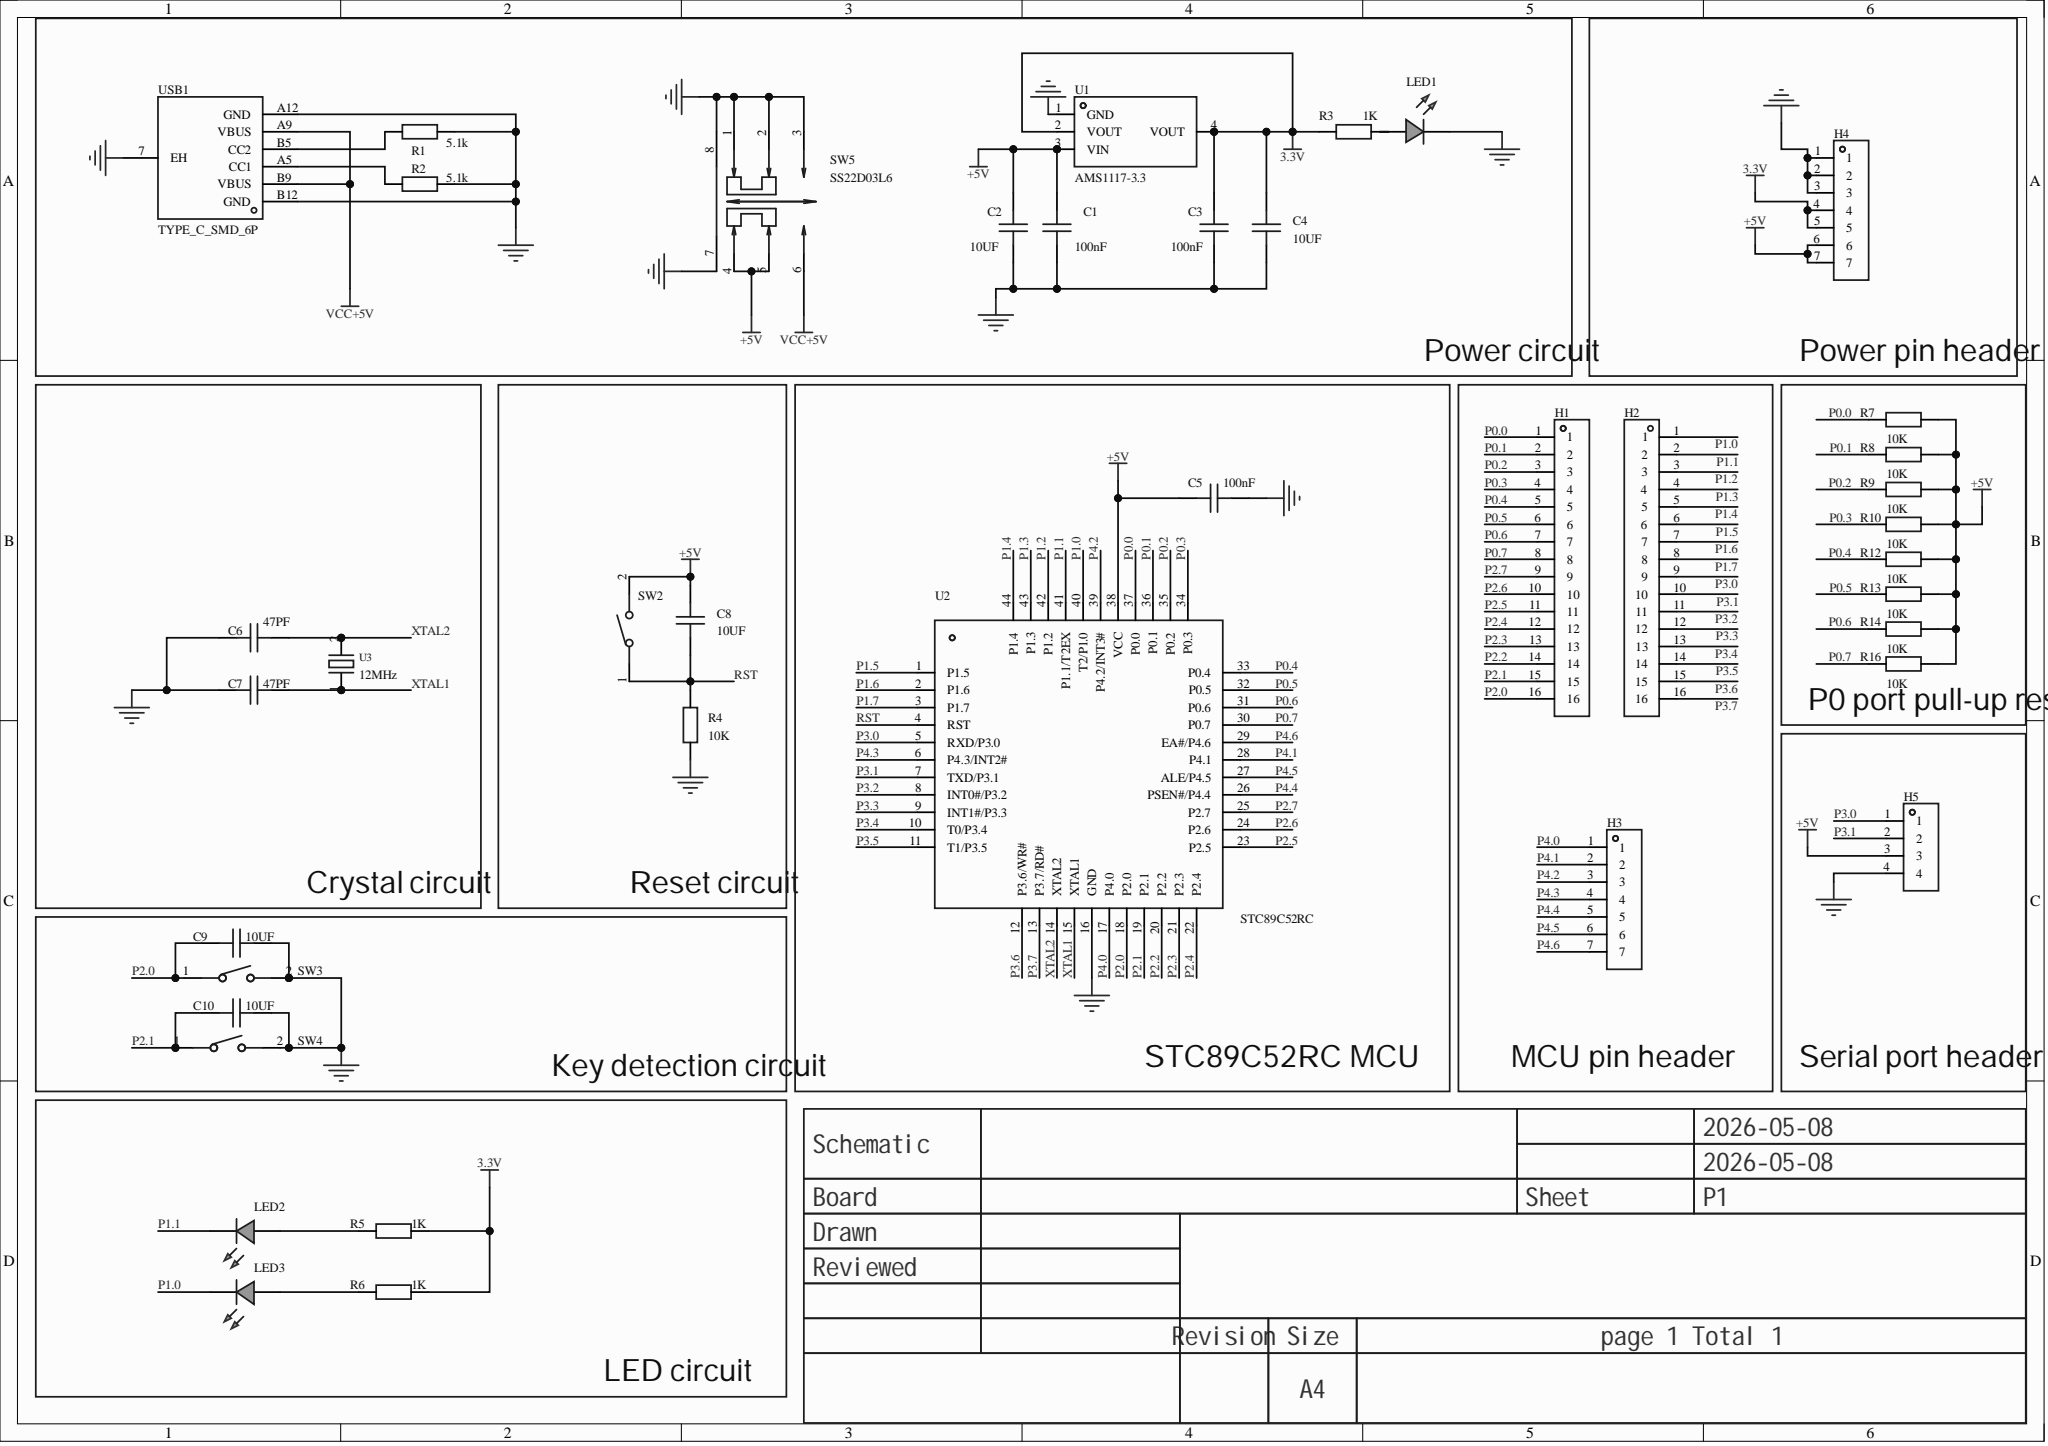Circuit board | Altium Designer | 40 parts | 51 nets
Bill of materials:
Comment,Description,Designator,Footprint,LibRef,Quantity
"100nF","","C1, C3, C5","C0805","CAP_0805","3"
"10UF","","C2, C4, C8, C9, C10","C0805","CAP_0805","5"
"47PF","","C6, C7","C0805","CAP_0805","2"
"","Pitch: 2.54mm; Total pins: 16; Rows: 1; Pin structure: 1x16P; Row spacing: -; Mounting type: Through-hole; Round/square pin: Square; Rated current: 3A; Rated voltage: -; Mating pin length: 6mm; Plastic height: 2.5mm; Termination pin length: 3mm; Contact material: -; Operating temp: -40℃~+105℃; Color: Black;","H1, H2","HDR-TH_16P-P2.54-V-M","HDR-M_2.54_1x16P","2"
"","","H3, H4","HDR-TH_7P-P2.54-V-M","HDR-M_2.54_1x7P","2"
"","","H5","HDR-TH_4P-P2.54-V-M","HDR-M_2.54_1x4P","1"
"","","LED1, LED2, LED3","LED_0805","LED_0805-G","3"
"5.1k","","R1, R2","R0805","Res_0805","2"
"1K","","R3","R0603","Res_0603","1"
"10K","","R4, R7, R8, R9, R10, R12, R13, R14, R16","R0805","Res_0805","9"
"1K","","R5, R6","R0805","Res_0805","2"
"Tact switch 3*4*H","","SW2, SW3, SW4","SW-SMD_L4.0-W2.9-LS5.0","轻触按键3*4*H","3"
"SS22D03L6","Circuit: DPDT; Mounting: Through-hole; Switch color: Black; Rated current (DC): 300mA; Rated voltage (DC): 50V; Rated current (AC): 300mA; Rated voltage (AC): 50V; Mechanical life: 1万次;","SW5","SW-TH_SS-22D03-L4","SS22D03L6","1"
"AMS1117-3.3","Output type: Fixed; Max input voltage: -; Output voltage: 3.3V; Max output current: 1A; PSRR: 72dB@(120Hz); Output polarity: Positive;","U1","SOT-223-3_L6.5-W3.4-P2.30-LS7.0-BR","AMS1117-3.3_C6186","1"
"STC89C52RC","CPU core: 51 series; Program memory: 8KB; RAM total: 512Byte; GPIO ports: 39; Operating voltage: 3.3V~5.5V; Max CPU frequency: -; Program memory type: FLASH;","U2","LQFP-44_L10.0-W10.0-P0.80-LS12.0-BL","STC89C52RC-40I-LQFP44","1"
"12MHz","Frequency: 12MHz; Frequency deviation at room temp: ±30ppm; Load capacitance: 18pF; Frequency stability (full temp): ±35ppm;","U3","CRYSTAL-SMD_L11.4-W4.7-LS12.7","ABLS-12.000MHZ-B4H-T","1"
"TYPE_C_SMD_6P","","USB1","TYPE-C-SMD_TYPE-C-6P","TYPE_C_SMD_6P","1"
Netlist (Protel format):
[
C1
C0805
100nF



]
[
C2
C0805
10UF



]
[
C3
C0805
100nF



]
[
C4
C0805
10UF



]
[
C5
C0805
100nF



]
[
C6
C0805
47PF



]
[
C7
C0805
47PF



]
[
C8
C0805
10UF



]
[
C9
C0805
10UF



]
[
C10
C0805
10UF



]
[
H1
HDR-TH_16P-P2.54-V-M




]
[
H2
HDR-TH_16P-P2.54-V-M




]
[
H3
HDR-TH_7P-P2.54-V-M




]
[
H4
HDR-TH_7P-P2.54-V-M




]
[
H5
HDR-TH_4P-P2.54-V-M




]
[
LED1
LED_0805




]
[
LED2
LED_0805




]
[
LED3
LED_0805




]
[
R1
R0805
5.1k



]
[
R2
R0805
5.1k



]
[
R3
R0603
1K



]
[
R4
R0805
10K



]
[
R5
R0805
1K



]
[
R6
R0805
1K



]
[
R7
R0805
10K



]
[
R8
R0805
10K



]
[
R9
R0805
10K



]
[
R10
R0805
10K



]
[
R12
R0805
10K



]
[
R13
R0805
10K



]
[
R14
R0805
10K



]
[
R16
R0805
10K



]
[
SW2
SW-SMD_L4.0-W2.9-LS5.0
Tact switch 3*4*H



]
[
SW3
SW-SMD_L4.0-W2.9-LS5.0
Tact switch 3*4*H



]
[
SW4
SW-SMD_L4.0-W2.9-LS5.0
Tact switch 3*4*H



]
[
SW5
SW-TH_SS-22D03-L4
SS22D03L6



]
[
U1
SOT-223-3_L6.5-W3.4-P2.30-LS7.0-BR
AMS1117-3.3



]
[
U2
LQFP-44_L10.0-W10.0-P0.80-LS12.0-BL
STC89C52RC



]
[
U3
CRYSTAL-SMD_L11.4-W4.7-LS12.7
12MHz



]
[
USB1
TYPE-C-SMD_TYPE-C-6P
TYPE_C_SMD_6P



]
(
XTAL2
C6-1
U2-14
U3-2
)
(
XTAL1
C7-1
U2-15
U3-1
)
(
VCC+5V
SW5-6
USB1-A9
USB1-B9
)
(
RST
C8-2
R4-2
SW2-1
U2-4
)
(
P4.6
H3-7
U2-29
)
(
P4.5
H3-6
U2-27
)
(
P4.4
H3-5
U2-26
)
(
P4.3
H3-4
U2-6
)
(
P4.2
H3-3
U2-39
)
(
P4.1
H3-2
U2-28
)
(
P4.0
H3-1
U2-17
)
(
P3.7
H2-16
U2-13
)
(
P3.6
H2-15
U2-12
)
(
P3.5
H2-14
U2-11
)
(
P3.4
H2-13
U2-10
)
(
P3.3
H2-12
U2-9
)
(
P3.2
H2-11
U2-8
)
(
P3.1
H2-10
H5-2
U2-7
)
(
P3.0
H2-9
H5-1
U2-5
)
(
P2.7
H1-9
U2-25
)
(
P2.6
H1-10
U2-24
)
(
P2.5
H1-11
U2-23
)
(
P2.4
H1-12
U2-22
)
(
P2.3
H1-13
U2-21
)
(
P2.2
H1-14
U2-20
)
(
P2.1
C10-2
H1-15
SW4-1
U2-19
)
(
P2.0
C9-2
H1-16
SW3-1
U2-18
)
(
P1.7
H2-8
U2-3
)
(
P1.6
H2-7
U2-2
)
(
P1.5
H2-6
U2-1
)
(
P1.4
H2-5
U2-44
)
(
P1.3
H2-4
U2-43
)
(
P1.2
H2-3
U2-42
)
(
P1.1
H2-2
LED2-1
U2-41
)
(
P1.0
H2-1
LED3-1
U2-40
)
(
P0.7
H1-8
R16-2
U2-30
)
(
P0.6
H1-7
R14-2
U2-31
)
(
P0.5
H1-6
R13-2
U2-32
)
(
P0.4
H1-5
R12-2
U2-33
)
(
P0.3
H1-4
R10-2
U2-34
)
(
P0.2
H1-3
R9-2
U2-35
)
(
P0.1
H1-2
R8-2
U2-36
)
(
P0.0
H1-1
R7-2
U2-37
)
(
NetR2_1
R2-1
USB1-A5
)
(
NetR1_1
R1-1
USB1-B5
)
(
NetLED3_2
LED3-2
R6-1
)
(
NetLED2_2
LED2-2
R5-1
)
(
NetLED1_2
LED1-2
R3-2
)
(
GND
C1-1
C2-1
C3-1
C4-1
C5-1
C6-2
C7-2
C9-1
C10-1
H4-1
H4-2
H4-3
H5-4
LED1-1
R1-2
R2-2
R4-1
SW3-2
SW4-2
SW5-1
SW5-2
SW5-3
SW5-7
SW5-8
U1-1
U2-16
USB1-7
USB1-A12
USB1-B12
)
(
+5V
C1-2
C2-2
C5-2
C8-1
H4-6
H4-7
H5-3
R7-1
R8-1
R9-1
R10-1
R12-1
R13-1
R14-1
R16-1
SW2-2
SW5-4
SW5-5
U1-3
U2-38
)
(
3.3V
C3-2
C4-2
H4-4
H4-5
R3-1
R5-2
R6-2
U1-2
U1-4
)